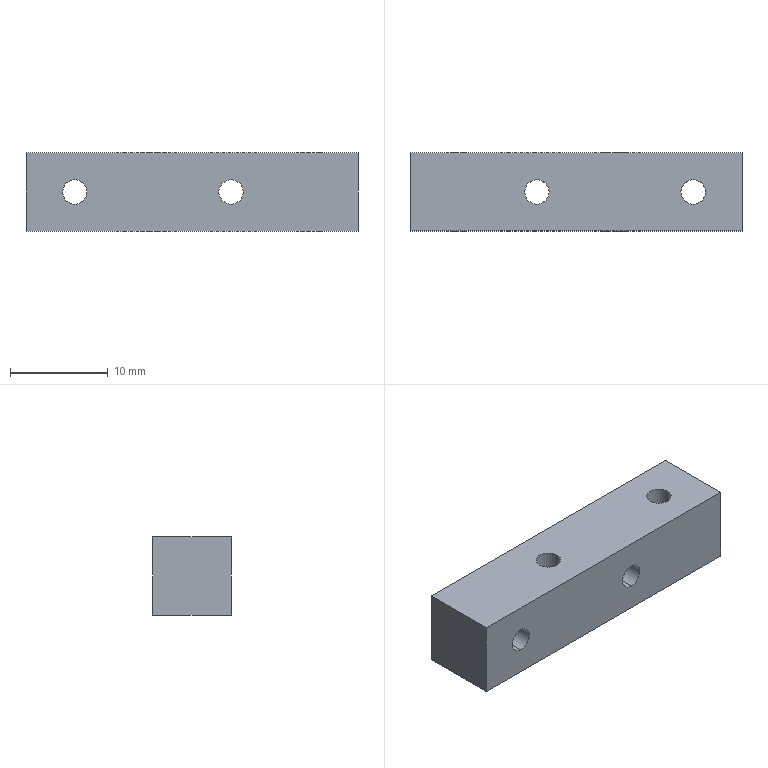Part | SolidWorks | features HoleWzd 2, Extrusion 1 | 1 solid | 14 faces | box 34 x 8 x 8 mm | volume 2019 mm3 | cylinder 8 | plane 6 | commonest cylinder face diameters 2.5 x8
STEP:
#1=CARTESIAN_POINT('',(-5.25,4.,-4.));
#2=VERTEX_POINT('',#1);
#3=CARTESIAN_POINT('',(-2.75,4.,-4.));
#4=VERTEX_POINT('',#3);
#5=CARTESIAN_POINT('',(-4.,4.,-4.));
#6=DIRECTION('',(0.,0.,1.));
#7=DIRECTION('',(1.,0.,0.));
#8=AXIS2_PLACEMENT_3D('',#5,#6,#7);
#9=CIRCLE('',#8,1.25);
#10=EDGE_CURVE('',#2,#4,#9,.T.);
#11=ORIENTED_EDGE('',*,*,#10,.F.);
#12=CARTESIAN_POINT('',(-5.25,4.,4.));
#13=VERTEX_POINT('',#12);
#14=CARTESIAN_POINT('',(-5.25,4.,4.));
#15=DIRECTION('',(0.,0.,1.));
#16=VECTOR('',#15,1000.);
#17=LINE('',#14,#16);
#18=EDGE_CURVE('',#2,#13,#17,.T.);
#19=ORIENTED_EDGE('',*,*,#18,.T.);
#20=CARTESIAN_POINT('',(-2.75,4.,4.));
#21=VERTEX_POINT('',#20);
#22=CARTESIAN_POINT('',(-4.,4.,4.));
#23=DIRECTION('',(0.,0.,1.));
#24=DIRECTION('',(1.,0.,0.));
#25=AXIS2_PLACEMENT_3D('',#22,#23,#24);
#26=CIRCLE('',#25,1.25);
#27=EDGE_CURVE('',#13,#21,#26,.T.);
#28=ORIENTED_EDGE('',*,*,#27,.T.);
#29=CARTESIAN_POINT('',(-2.75,4.,4.));
#30=DIRECTION('',(0.,0.,1.));
#31=VECTOR('',#30,1000.);
#32=LINE('',#29,#31);
#33=EDGE_CURVE('',#4,#21,#32,.T.);
#34=ORIENTED_EDGE('',*,*,#33,.F.);
#35=EDGE_LOOP('',(#11,#19,#28,#34));
#36=FACE_OUTER_BOUND('',#35,.T.);
#37=CARTESIAN_POINT('',(-4.,4.,4.));
#38=DIRECTION('',(0.,0.,1.));
#39=DIRECTION('',(1.,0.,0.));
#40=AXIS2_PLACEMENT_3D('',#37,#38,#39);
#41=CYLINDRICAL_SURFACE('',#40,1.25);
#42=ADVANCED_FACE('',(#36),#41,.F.);
#43=CARTESIAN_POINT('',(10.75,4.,-4.));
#44=VERTEX_POINT('',#43);
#45=CARTESIAN_POINT('',(13.25,4.,-4.));
#46=VERTEX_POINT('',#45);
#47=CARTESIAN_POINT('',(12.,4.,-4.));
#48=DIRECTION('',(0.,0.,1.));
#49=DIRECTION('',(1.,0.,0.));
#50=AXIS2_PLACEMENT_3D('',#47,#48,#49);
#51=CIRCLE('',#50,1.25);
#52=EDGE_CURVE('',#44,#46,#51,.T.);
#53=ORIENTED_EDGE('',*,*,#52,.F.);
#54=CARTESIAN_POINT('',(10.75,4.,4.));
#55=VERTEX_POINT('',#54);
#56=CARTESIAN_POINT('',(10.75,4.,4.));
#57=DIRECTION('',(0.,0.,1.));
#58=VECTOR('',#57,1000.);
#59=LINE('',#56,#58);
#60=EDGE_CURVE('',#44,#55,#59,.T.);
#61=ORIENTED_EDGE('',*,*,#60,.T.);
#62=CARTESIAN_POINT('',(13.25,4.,4.));
#63=VERTEX_POINT('',#62);
#64=CARTESIAN_POINT('',(12.,4.,4.));
#65=DIRECTION('',(0.,0.,1.));
#66=DIRECTION('',(1.,0.,0.));
#67=AXIS2_PLACEMENT_3D('',#64,#65,#66);
#68=CIRCLE('',#67,1.25);
#69=EDGE_CURVE('',#55,#63,#68,.T.);
#70=ORIENTED_EDGE('',*,*,#69,.T.);
#71=CARTESIAN_POINT('',(13.25,4.,4.));
#72=DIRECTION('',(0.,0.,1.));
#73=VECTOR('',#72,1000.);
#74=LINE('',#71,#73);
#75=EDGE_CURVE('',#46,#63,#74,.T.);
#76=ORIENTED_EDGE('',*,*,#75,.F.);
#77=EDGE_LOOP('',(#53,#61,#70,#76));
#78=FACE_OUTER_BOUND('',#77,.T.);
#79=CARTESIAN_POINT('',(12.,4.,4.));
#80=DIRECTION('',(0.,0.,1.));
#81=DIRECTION('',(1.,0.,0.));
#82=AXIS2_PLACEMENT_3D('',#79,#80,#81);
#83=CYLINDRICAL_SURFACE('',#82,1.25);
#84=ADVANCED_FACE('',(#78),#83,.F.);
#85=CARTESIAN_POINT('',(-12.,0.,-1.25));
#86=VERTEX_POINT('',#85);
#87=CARTESIAN_POINT('',(-12.,0.,1.25));
#88=VERTEX_POINT('',#87);
#89=CARTESIAN_POINT('',(-12.,0.,0.));
#90=DIRECTION('',(0.,1.,0.));
#91=DIRECTION('',(0.,0.,1.));
#92=AXIS2_PLACEMENT_3D('',#89,#90,#91);
#93=CIRCLE('',#92,1.25);
#94=EDGE_CURVE('',#86,#88,#93,.T.);
#95=ORIENTED_EDGE('',*,*,#94,.F.);
#96=CARTESIAN_POINT('',(-12.,8.,-1.25));
#97=VERTEX_POINT('',#96);
#98=CARTESIAN_POINT('',(-12.,8.,-1.25));
#99=DIRECTION('',(0.,1.,0.));
#100=VECTOR('',#99,1000.);
#101=LINE('',#98,#100);
#102=EDGE_CURVE('',#86,#97,#101,.T.);
#103=ORIENTED_EDGE('',*,*,#102,.T.);
#104=CARTESIAN_POINT('',(-12.,8.,1.25));
#105=VERTEX_POINT('',#104);
#106=CARTESIAN_POINT('',(-12.,8.,0.));
#107=DIRECTION('',(0.,1.,0.));
#108=DIRECTION('',(0.,0.,1.));
#109=AXIS2_PLACEMENT_3D('',#106,#107,#108);
#110=CIRCLE('',#109,1.25);
#111=EDGE_CURVE('',#97,#105,#110,.T.);
#112=ORIENTED_EDGE('',*,*,#111,.T.);
#113=CARTESIAN_POINT('',(-12.,8.,1.25));
#114=DIRECTION('',(0.,1.,0.));
#115=VECTOR('',#114,1000.);
#116=LINE('',#113,#115);
#117=EDGE_CURVE('',#88,#105,#116,.T.);
#118=ORIENTED_EDGE('',*,*,#117,.F.);
#119=EDGE_LOOP('',(#95,#103,#112,#118));
#120=FACE_OUTER_BOUND('',#119,.T.);
#121=CARTESIAN_POINT('',(-12.,8.,0.));
#122=DIRECTION('',(0.,1.,0.));
#123=DIRECTION('',(0.,0.,1.));
#124=AXIS2_PLACEMENT_3D('',#121,#122,#123);
#125=CYLINDRICAL_SURFACE('',#124,1.25);
#126=ADVANCED_FACE('',(#120),#125,.F.);
#127=CARTESIAN_POINT('',(4.,0.,-1.25));
#128=VERTEX_POINT('',#127);
#129=CARTESIAN_POINT('',(4.,0.,1.25));
#130=VERTEX_POINT('',#129);
#131=CARTESIAN_POINT('',(4.,0.,0.));
#132=DIRECTION('',(0.,1.,0.));
#133=DIRECTION('',(0.,0.,1.));
#134=AXIS2_PLACEMENT_3D('',#131,#132,#133);
#135=CIRCLE('',#134,1.25);
#136=EDGE_CURVE('',#128,#130,#135,.T.);
#137=ORIENTED_EDGE('',*,*,#136,.F.);
#138=CARTESIAN_POINT('',(4.,8.,-1.25));
#139=VERTEX_POINT('',#138);
#140=CARTESIAN_POINT('',(4.,8.,-1.25));
#141=DIRECTION('',(0.,1.,0.));
#142=VECTOR('',#141,1000.);
#143=LINE('',#140,#142);
#144=EDGE_CURVE('',#128,#139,#143,.T.);
#145=ORIENTED_EDGE('',*,*,#144,.T.);
#146=CARTESIAN_POINT('',(4.,8.,1.25));
#147=VERTEX_POINT('',#146);
#148=CARTESIAN_POINT('',(4.,8.,0.));
#149=DIRECTION('',(0.,1.,0.));
#150=DIRECTION('',(0.,0.,1.));
#151=AXIS2_PLACEMENT_3D('',#148,#149,#150);
#152=CIRCLE('',#151,1.25);
#153=EDGE_CURVE('',#139,#147,#152,.T.);
#154=ORIENTED_EDGE('',*,*,#153,.T.);
#155=CARTESIAN_POINT('',(4.,8.,1.25));
#156=DIRECTION('',(0.,1.,0.));
#157=VECTOR('',#156,1000.);
#158=LINE('',#155,#157);
#159=EDGE_CURVE('',#130,#147,#158,.T.);
#160=ORIENTED_EDGE('',*,*,#159,.F.);
#161=EDGE_LOOP('',(#137,#145,#154,#160));
#162=FACE_OUTER_BOUND('',#161,.T.);
#163=CARTESIAN_POINT('',(4.,8.,0.));
#164=DIRECTION('',(0.,1.,0.));
#165=DIRECTION('',(0.,0.,1.));
#166=AXIS2_PLACEMENT_3D('',#163,#164,#165);
#167=CYLINDRICAL_SURFACE('',#166,1.25);
#168=ADVANCED_FACE('',(#162),#167,.F.);
#169=CARTESIAN_POINT('',(17.,0.,4.));
#170=VERTEX_POINT('',#169);
#171=CARTESIAN_POINT('',(17.,0.,-4.));
#172=VERTEX_POINT('',#171);
#173=CARTESIAN_POINT('',(17.,0.,-4.));
#174=DIRECTION('',(0.,0.,-1.));
#175=VECTOR('',#174,1000.);
#176=LINE('',#173,#175);
#177=EDGE_CURVE('',#170,#172,#176,.T.);
#178=ORIENTED_EDGE('',*,*,#177,.T.);
#179=CARTESIAN_POINT('',(17.,8.,-4.));
#180=VERTEX_POINT('',#179);
#181=CARTESIAN_POINT('',(17.,8.,-4.));
#182=DIRECTION('',(0.,-1.,0.));
#183=VECTOR('',#182,1000.);
#184=LINE('',#181,#183);
#185=EDGE_CURVE('',#180,#172,#184,.T.);
#186=ORIENTED_EDGE('',*,*,#185,.F.);
#187=CARTESIAN_POINT('',(17.,8.,4.));
#188=VERTEX_POINT('',#187);
#189=CARTESIAN_POINT('',(17.,8.,-4.));
#190=DIRECTION('',(0.,0.,-1.));
#191=VECTOR('',#190,1000.);
#192=LINE('',#189,#191);
#193=EDGE_CURVE('',#188,#180,#192,.T.);
#194=ORIENTED_EDGE('',*,*,#193,.F.);
#195=CARTESIAN_POINT('',(17.,8.,4.));
#196=DIRECTION('',(0.,-1.,0.));
#197=VECTOR('',#196,1000.);
#198=LINE('',#195,#197);
#199=EDGE_CURVE('',#188,#170,#198,.T.);
#200=ORIENTED_EDGE('',*,*,#199,.T.);
#201=EDGE_LOOP('',(#178,#186,#194,#200));
#202=FACE_OUTER_BOUND('',#201,.T.);
#203=CARTESIAN_POINT('',(17.,8.,-4.));
#204=DIRECTION('',(-1.,0.,0.));
#205=DIRECTION('',(0.,0.,1.));
#206=AXIS2_PLACEMENT_3D('',#203,#204,#205);
#207=PLANE('',#206);
#208=ADVANCED_FACE('',(#202),#207,.F.);
#209=CARTESIAN_POINT('',(-4.,4.,-4.));
#210=DIRECTION('',(0.,0.,1.));
#211=DIRECTION('',(1.,0.,0.));
#212=AXIS2_PLACEMENT_3D('',#209,#210,#211);
#213=CIRCLE('',#212,1.25);
#214=EDGE_CURVE('',#4,#2,#213,.T.);
#215=ORIENTED_EDGE('',*,*,#214,.T.);
#216=ORIENTED_EDGE('',*,*,#10,.T.);
#217=EDGE_LOOP('',(#215,#216));
#218=FACE_BOUND('',#217,.T.);
#219=CARTESIAN_POINT('',(12.,4.,-4.));
#220=DIRECTION('',(0.,0.,1.));
#221=DIRECTION('',(1.,0.,0.));
#222=AXIS2_PLACEMENT_3D('',#219,#220,#221);
#223=CIRCLE('',#222,1.25);
#224=EDGE_CURVE('',#46,#44,#223,.T.);
#225=ORIENTED_EDGE('',*,*,#224,.T.);
#226=ORIENTED_EDGE('',*,*,#52,.T.);
#227=EDGE_LOOP('',(#225,#226));
#228=FACE_BOUND('',#227,.T.);
#229=CARTESIAN_POINT('',(-17.,0.,-4.));
#230=VERTEX_POINT('',#229);
#231=CARTESIAN_POINT('',(-17.,0.,-4.));
#232=DIRECTION('',(-1.,0.,0.));
#233=VECTOR('',#232,1000.);
#234=LINE('',#231,#233);
#235=EDGE_CURVE('',#172,#230,#234,.T.);
#236=ORIENTED_EDGE('',*,*,#235,.T.);
#237=CARTESIAN_POINT('',(-17.,8.,-4.));
#238=VERTEX_POINT('',#237);
#239=CARTESIAN_POINT('',(-17.,8.,-4.));
#240=DIRECTION('',(0.,-1.,0.));
#241=VECTOR('',#240,1000.);
#242=LINE('',#239,#241);
#243=EDGE_CURVE('',#238,#230,#242,.T.);
#244=ORIENTED_EDGE('',*,*,#243,.F.);
#245=CARTESIAN_POINT('',(-17.,8.,-4.));
#246=DIRECTION('',(-1.,0.,0.));
#247=VECTOR('',#246,1000.);
#248=LINE('',#245,#247);
#249=EDGE_CURVE('',#180,#238,#248,.T.);
#250=ORIENTED_EDGE('',*,*,#249,.F.);
#251=ORIENTED_EDGE('',*,*,#185,.T.);
#252=EDGE_LOOP('',(#236,#244,#250,#251));
#253=FACE_OUTER_BOUND('',#252,.T.);
#254=CARTESIAN_POINT('',(-17.,8.,-4.));
#255=DIRECTION('',(0.,0.,1.));
#256=DIRECTION('',(1.,0.,0.));
#257=AXIS2_PLACEMENT_3D('',#254,#255,#256);
#258=PLANE('',#257);
#259=ADVANCED_FACE('',(#218,#228,#253),#258,.F.);
#260=CARTESIAN_POINT('',(-17.,0.,4.));
#261=VERTEX_POINT('',#260);
#262=CARTESIAN_POINT('',(-17.,0.,-4.));
#263=DIRECTION('',(0.,0.,1.));
#264=VECTOR('',#263,1000.);
#265=LINE('',#262,#264);
#266=EDGE_CURVE('',#230,#261,#265,.T.);
#267=ORIENTED_EDGE('',*,*,#266,.T.);
#268=CARTESIAN_POINT('',(-17.,8.,4.));
#269=VERTEX_POINT('',#268);
#270=CARTESIAN_POINT('',(-17.,8.,4.));
#271=DIRECTION('',(0.,-1.,0.));
#272=VECTOR('',#271,1000.);
#273=LINE('',#270,#272);
#274=EDGE_CURVE('',#269,#261,#273,.T.);
#275=ORIENTED_EDGE('',*,*,#274,.F.);
#276=CARTESIAN_POINT('',(-17.,8.,-4.));
#277=DIRECTION('',(0.,0.,1.));
#278=VECTOR('',#277,1000.);
#279=LINE('',#276,#278);
#280=EDGE_CURVE('',#238,#269,#279,.T.);
#281=ORIENTED_EDGE('',*,*,#280,.F.);
#282=ORIENTED_EDGE('',*,*,#243,.T.);
#283=EDGE_LOOP('',(#267,#275,#281,#282));
#284=FACE_OUTER_BOUND('',#283,.T.);
#285=CARTESIAN_POINT('',(-17.,8.,-4.));
#286=DIRECTION('',(1.,0.,0.));
#287=DIRECTION('',(0.,0.,-1.));
#288=AXIS2_PLACEMENT_3D('',#285,#286,#287);
#289=PLANE('',#288);
#290=ADVANCED_FACE('',(#284),#289,.F.);
#291=CARTESIAN_POINT('',(-4.,4.,4.));
#292=DIRECTION('',(0.,0.,1.));
#293=DIRECTION('',(1.,0.,0.));
#294=AXIS2_PLACEMENT_3D('',#291,#292,#293);
#295=CIRCLE('',#294,1.25);
#296=EDGE_CURVE('',#21,#13,#295,.T.);
#297=ORIENTED_EDGE('',*,*,#296,.F.);
#298=ORIENTED_EDGE('',*,*,#27,.F.);
#299=EDGE_LOOP('',(#297,#298));
#300=FACE_BOUND('',#299,.T.);
#301=CARTESIAN_POINT('',(12.,4.,4.));
#302=DIRECTION('',(0.,0.,1.));
#303=DIRECTION('',(1.,0.,0.));
#304=AXIS2_PLACEMENT_3D('',#301,#302,#303);
#305=CIRCLE('',#304,1.25);
#306=EDGE_CURVE('',#63,#55,#305,.T.);
#307=ORIENTED_EDGE('',*,*,#306,.F.);
#308=ORIENTED_EDGE('',*,*,#69,.F.);
#309=EDGE_LOOP('',(#307,#308));
#310=FACE_BOUND('',#309,.T.);
#311=CARTESIAN_POINT('',(-17.,0.,4.));
#312=DIRECTION('',(1.,0.,0.));
#313=VECTOR('',#312,1000.);
#314=LINE('',#311,#313);
#315=EDGE_CURVE('',#261,#170,#314,.T.);
#316=ORIENTED_EDGE('',*,*,#315,.T.);
#317=ORIENTED_EDGE('',*,*,#199,.F.);
#318=CARTESIAN_POINT('',(-17.,8.,4.));
#319=DIRECTION('',(1.,0.,0.));
#320=VECTOR('',#319,1000.);
#321=LINE('',#318,#320);
#322=EDGE_CURVE('',#269,#188,#321,.T.);
#323=ORIENTED_EDGE('',*,*,#322,.F.);
#324=ORIENTED_EDGE('',*,*,#274,.T.);
#325=EDGE_LOOP('',(#316,#317,#323,#324));
#326=FACE_OUTER_BOUND('',#325,.T.);
#327=CARTESIAN_POINT('',(-17.,8.,4.));
#328=DIRECTION('',(0.,0.,-1.));
#329=DIRECTION('',(-1.,0.,0.));
#330=AXIS2_PLACEMENT_3D('',#327,#328,#329);
#331=PLANE('',#330);
#332=ADVANCED_FACE('',(#300,#310,#326),#331,.F.);
#333=CARTESIAN_POINT('',(-12.,8.,0.));
#334=DIRECTION('',(0.,1.,0.));
#335=DIRECTION('',(0.,0.,1.));
#336=AXIS2_PLACEMENT_3D('',#333,#334,#335);
#337=CIRCLE('',#336,1.25);
#338=EDGE_CURVE('',#105,#97,#337,.T.);
#339=ORIENTED_EDGE('',*,*,#338,.F.);
#340=ORIENTED_EDGE('',*,*,#111,.F.);
#341=EDGE_LOOP('',(#339,#340));
#342=FACE_BOUND('',#341,.T.);
#343=CARTESIAN_POINT('',(4.,8.,0.));
#344=DIRECTION('',(0.,1.,0.));
#345=DIRECTION('',(0.,0.,1.));
#346=AXIS2_PLACEMENT_3D('',#343,#344,#345);
#347=CIRCLE('',#346,1.25);
#348=EDGE_CURVE('',#147,#139,#347,.T.);
#349=ORIENTED_EDGE('',*,*,#348,.F.);
#350=ORIENTED_EDGE('',*,*,#153,.F.);
#351=EDGE_LOOP('',(#349,#350));
#352=FACE_BOUND('',#351,.T.);
#353=ORIENTED_EDGE('',*,*,#193,.T.);
#354=ORIENTED_EDGE('',*,*,#249,.T.);
#355=ORIENTED_EDGE('',*,*,#280,.T.);
#356=ORIENTED_EDGE('',*,*,#322,.T.);
#357=EDGE_LOOP('',(#353,#354,#355,#356));
#358=FACE_OUTER_BOUND('',#357,.T.);
#359=CARTESIAN_POINT('',(0.,8.,0.));
#360=DIRECTION('',(0.,1.,0.));
#361=DIRECTION('',(0.,0.,1.));
#362=AXIS2_PLACEMENT_3D('',#359,#360,#361);
#363=PLANE('',#362);
#364=ADVANCED_FACE('',(#342,#352,#358),#363,.T.);
#365=CARTESIAN_POINT('',(-12.,0.,0.));
#366=DIRECTION('',(0.,1.,0.));
#367=DIRECTION('',(0.,0.,1.));
#368=AXIS2_PLACEMENT_3D('',#365,#366,#367);
#369=CIRCLE('',#368,1.25);
#370=EDGE_CURVE('',#88,#86,#369,.T.);
#371=ORIENTED_EDGE('',*,*,#370,.T.);
#372=ORIENTED_EDGE('',*,*,#94,.T.);
#373=EDGE_LOOP('',(#371,#372));
#374=FACE_BOUND('',#373,.T.);
#375=CARTESIAN_POINT('',(4.,0.,0.));
#376=DIRECTION('',(0.,1.,0.));
#377=DIRECTION('',(0.,0.,1.));
#378=AXIS2_PLACEMENT_3D('',#375,#376,#377);
#379=CIRCLE('',#378,1.25);
#380=EDGE_CURVE('',#130,#128,#379,.T.);
#381=ORIENTED_EDGE('',*,*,#380,.T.);
#382=ORIENTED_EDGE('',*,*,#136,.T.);
#383=EDGE_LOOP('',(#381,#382));
#384=FACE_BOUND('',#383,.T.);
#385=ORIENTED_EDGE('',*,*,#177,.F.);
#386=ORIENTED_EDGE('',*,*,#315,.F.);
#387=ORIENTED_EDGE('',*,*,#266,.F.);
#388=ORIENTED_EDGE('',*,*,#235,.F.);
#389=EDGE_LOOP('',(#385,#386,#387,#388));
#390=FACE_OUTER_BOUND('',#389,.T.);
#391=CARTESIAN_POINT('',(0.,0.,0.));
#392=DIRECTION('',(0.,1.,0.));
#393=DIRECTION('',(0.,0.,1.));
#394=AXIS2_PLACEMENT_3D('',#391,#392,#393);
#395=PLANE('',#394);
#396=ADVANCED_FACE('',(#374,#384,#390),#395,.F.);
#397=ORIENTED_EDGE('',*,*,#144,.F.);
#398=ORIENTED_EDGE('',*,*,#380,.F.);
#399=ORIENTED_EDGE('',*,*,#159,.T.);
#400=ORIENTED_EDGE('',*,*,#348,.T.);
#401=EDGE_LOOP('',(#397,#398,#399,#400));
#402=FACE_OUTER_BOUND('',#401,.T.);
#403=CARTESIAN_POINT('',(4.,8.,0.));
#404=DIRECTION('',(0.,1.,0.));
#405=DIRECTION('',(0.,0.,1.));
#406=AXIS2_PLACEMENT_3D('',#403,#404,#405);
#407=CYLINDRICAL_SURFACE('',#406,1.25);
#408=ADVANCED_FACE('',(#402),#407,.F.);
#409=ORIENTED_EDGE('',*,*,#102,.F.);
#410=ORIENTED_EDGE('',*,*,#370,.F.);
#411=ORIENTED_EDGE('',*,*,#117,.T.);
#412=ORIENTED_EDGE('',*,*,#338,.T.);
#413=EDGE_LOOP('',(#409,#410,#411,#412));
#414=FACE_OUTER_BOUND('',#413,.T.);
#415=CARTESIAN_POINT('',(-12.,8.,0.));
#416=DIRECTION('',(0.,1.,0.));
#417=DIRECTION('',(0.,0.,1.));
#418=AXIS2_PLACEMENT_3D('',#415,#416,#417);
#419=CYLINDRICAL_SURFACE('',#418,1.25);
#420=ADVANCED_FACE('',(#414),#419,.F.);
#421=ORIENTED_EDGE('',*,*,#60,.F.);
#422=ORIENTED_EDGE('',*,*,#224,.F.);
#423=ORIENTED_EDGE('',*,*,#75,.T.);
#424=ORIENTED_EDGE('',*,*,#306,.T.);
#425=EDGE_LOOP('',(#421,#422,#423,#424));
#426=FACE_OUTER_BOUND('',#425,.T.);
#427=CARTESIAN_POINT('',(12.,4.,4.));
#428=DIRECTION('',(0.,0.,1.));
#429=DIRECTION('',(1.,0.,0.));
#430=AXIS2_PLACEMENT_3D('',#427,#428,#429);
#431=CYLINDRICAL_SURFACE('',#430,1.25);
#432=ADVANCED_FACE('',(#426),#431,.F.);
#433=ORIENTED_EDGE('',*,*,#18,.F.);
#434=ORIENTED_EDGE('',*,*,#214,.F.);
#435=ORIENTED_EDGE('',*,*,#33,.T.);
#436=ORIENTED_EDGE('',*,*,#296,.T.);
#437=EDGE_LOOP('',(#433,#434,#435,#436));
#438=FACE_OUTER_BOUND('',#437,.T.);
#439=CARTESIAN_POINT('',(-4.,4.,4.));
#440=DIRECTION('',(0.,0.,1.));
#441=DIRECTION('',(1.,0.,0.));
#442=AXIS2_PLACEMENT_3D('',#439,#440,#441);
#443=CYLINDRICAL_SURFACE('',#442,1.25);
#444=ADVANCED_FACE('',(#438),#443,.F.);
#445=CLOSED_SHELL('',(#42,#84,#126,#168,#208,#259,#290,#332,#364,#396,#408,#420,#432,#444));
#446=MANIFOLD_SOLID_BREP('',#445);
#447=CARTESIAN_POINT('',(0.,0.,0.));
#448=DIRECTION('',(0.,0.,1.));
#449=DIRECTION('',(1.,0.,0.));
#450=AXIS2_PLACEMENT_3D('',#447,#448,#449);
#451=(LENGTH_UNIT()NAMED_UNIT(*)SI_UNIT(.MILLI.,.METRE.));
#452=UNCERTAINTY_MEASURE_WITH_UNIT(LENGTH_MEASURE(0.00001),#451,'','');
#453=(NAMED_UNIT(*)PLANE_ANGLE_UNIT()SI_UNIT($,.RADIAN.));
#454=(NAMED_UNIT(*)SI_UNIT($,.STERADIAN.)SOLID_ANGLE_UNIT());
#455=(GEOMETRIC_REPRESENTATION_CONTEXT(3)GLOBAL_UNCERTAINTY_ASSIGNED_CONTEXT((#452))GLOBAL_UNIT_ASSIGNED_CONTEXT((#451,#453,#454))REPRESENTATION_CONTEXT('',''));
#456=ADVANCED_BREP_SHAPE_REPRESENTATION('',(#446,#450),#455);